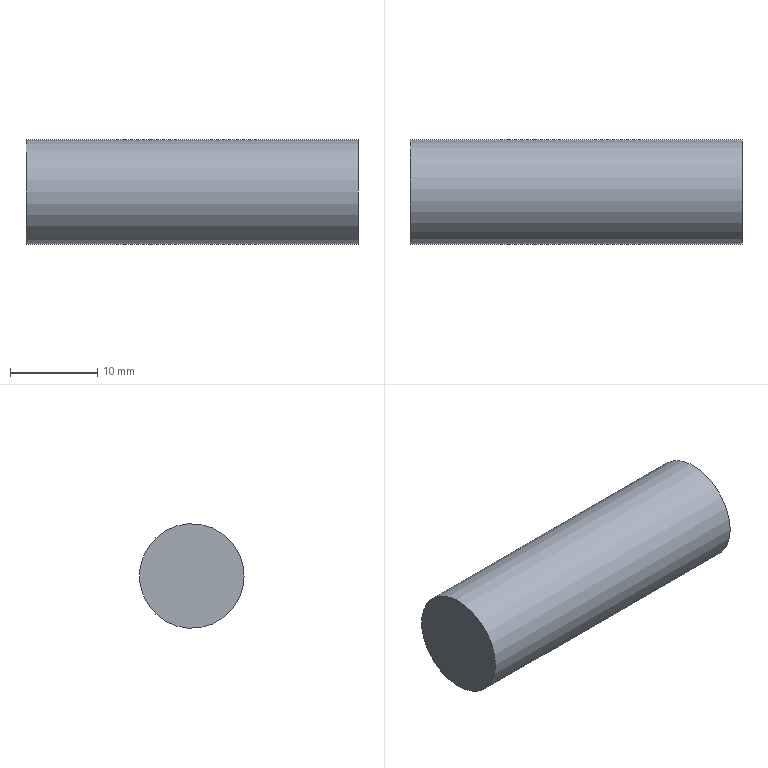Part | NX | features solid 2 | 1 solid | 3 faces | box 38.1 x 12 x 12 mm | volume 4309 mm3 | plane 2 | cylinder 1 | commonest cylinder face diameters 12 x1
STEP:
#1=CARTESIAN_POINT('',(-115.4,-99.5,-140.));
#2=VERTEX_POINT('',#1);
#3=CARTESIAN_POINT('',(-115.4,-93.5,-140.));
#4=DIRECTION('',(-1.,0.,0.));
#5=DIRECTION('',(0.,-1.,0.));
#6=AXIS2_PLACEMENT_3D('',#3,#4,#5);
#7=CIRCLE('',#6,6.);
#8=EDGE_CURVE('',#2,#2,#7,.T.);
#9=ORIENTED_EDGE('',*,*,#8,.T.);
#10=EDGE_LOOP('',(#9));
#11=FACE_BOUND('',#10,.T.);
#12=CARTESIAN_POINT('',(-153.5,-99.5,-140.));
#13=VERTEX_POINT('',#12);
#14=CARTESIAN_POINT('',(-153.5,-93.5,-140.));
#15=DIRECTION('',(-1.,0.,0.));
#16=DIRECTION('',(0.,-1.,0.));
#17=AXIS2_PLACEMENT_3D('',#14,#15,#16);
#18=CIRCLE('',#17,6.);
#19=EDGE_CURVE('',#13,#13,#18,.T.);
#20=ORIENTED_EDGE('',*,*,#19,.F.);
#21=EDGE_LOOP('',(#20));
#22=FACE_BOUND('',#21,.T.);
#23=CARTESIAN_POINT('',(-115.4,-93.5,-140.));
#24=DIRECTION('',(-1.,0.,0.));
#25=DIRECTION('',(0.,1.,0.));
#26=AXIS2_PLACEMENT_3D('',#23,#24,#25);
#27=CYLINDRICAL_SURFACE('',#26,6.);
#28=ADVANCED_FACE('',(#11,#22),#27,.T.);
#29=ORIENTED_EDGE('',*,*,#8,.F.);
#30=EDGE_LOOP('',(#29));
#31=FACE_BOUND('',#30,.T.);
#32=CARTESIAN_POINT('',(-115.4,-93.5,-140.));
#33=DIRECTION('',(1.,0.,0.));
#34=DIRECTION('',(0.,-1.,0.));
#35=AXIS2_PLACEMENT_3D('',#32,#33,#34);
#36=PLANE('',#35);
#37=ADVANCED_FACE('',(#31),#36,.T.);
#38=ORIENTED_EDGE('',*,*,#19,.T.);
#39=EDGE_LOOP('',(#38));
#40=FACE_BOUND('',#39,.T.);
#41=CARTESIAN_POINT('',(-153.5,-93.5,-140.));
#42=DIRECTION('',(1.,0.,0.));
#43=DIRECTION('',(0.,-1.,0.));
#44=AXIS2_PLACEMENT_3D('',#41,#42,#43);
#45=PLANE('',#44);
#46=ADVANCED_FACE('',(#40),#45,.F.);
#47=CLOSED_SHELL('',(#28,#37,#46));
#48=MANIFOLD_SOLID_BREP('',#47);
#49=(LENGTH_UNIT()NAMED_UNIT(*)SI_UNIT(.MILLI.,.METRE.));
#50=UNCERTAINTY_MEASURE_WITH_UNIT(LENGTH_MEASURE(0.00001),#49,'','');
#51=(NAMED_UNIT(*)PLANE_ANGLE_UNIT()SI_UNIT($,.RADIAN.));
#52=(NAMED_UNIT(*)SI_UNIT($,.STERADIAN.)SOLID_ANGLE_UNIT());
#53=(GEOMETRIC_REPRESENTATION_CONTEXT(3)GLOBAL_UNCERTAINTY_ASSIGNED_CONTEXT((#50))GLOBAL_UNIT_ASSIGNED_CONTEXT((#49,#51,#52))REPRESENTATION_CONTEXT('',''));
#54=ADVANCED_BREP_SHAPE_REPRESENTATION('',(#48),#53);